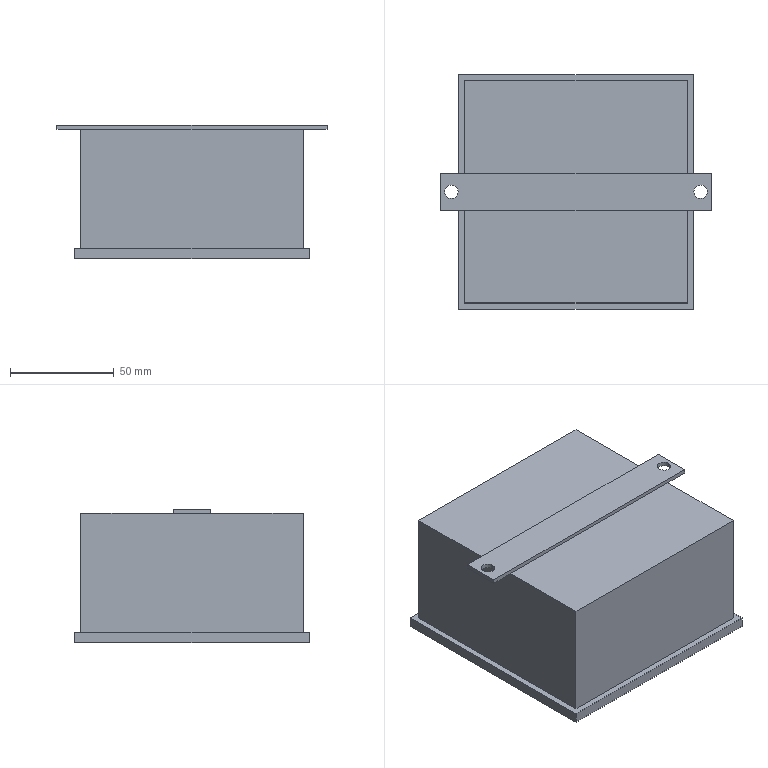Part | STEP file | DTC13-Tension control panel-Taimake | 1 solid | 112 faces | box 130 x 113 x 64.4 mm | volume 725565 mm3 | plane 60 | spline 48 | cylinder 4 | commonest cylinder face diameters 6.5 x4